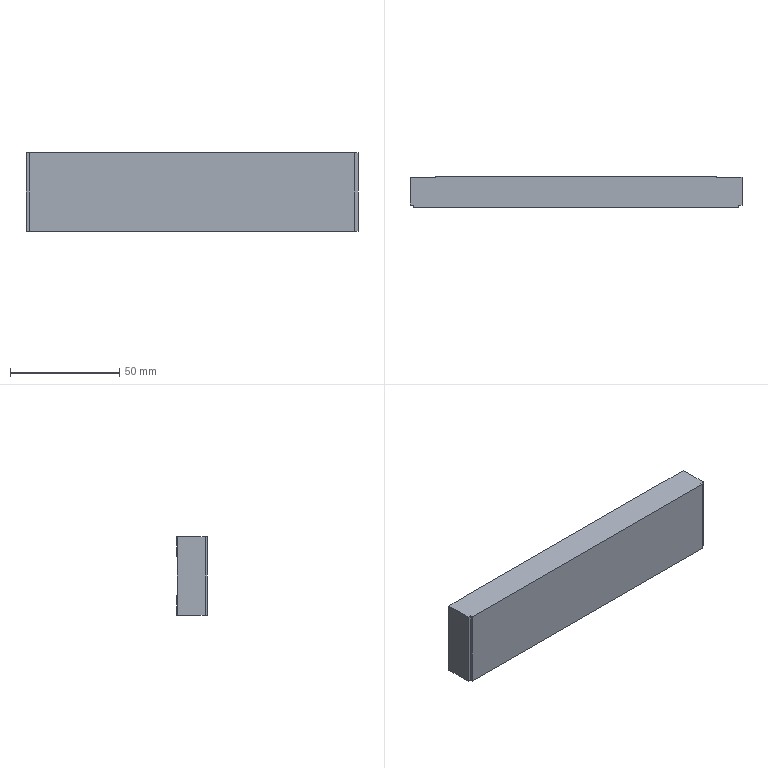Part | STEP file | HI_PRF40500s | 1 solid | 82 faces | box 152 x 14 x 36 mm | volume 74599 mm3 | plane 50 | cylinder 16 | cone 16 | commonest cylinder face diameters 4.917 x8 6 x8